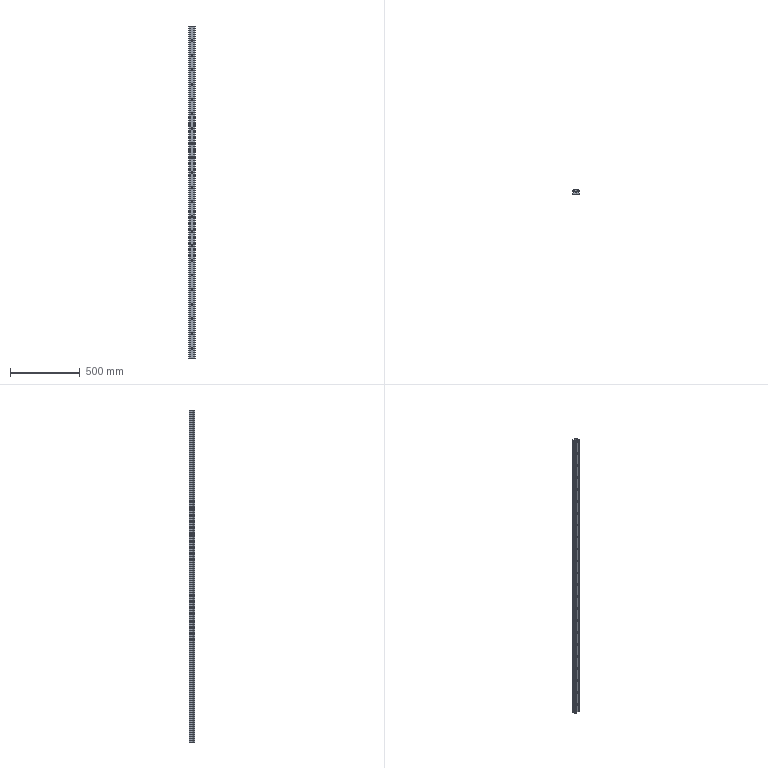Part | SolidWorks | features ICE 3, LPattern 2, BaseBody 1, RevCut 1 | 1 solid | 158 faces | box 45 x 38 x 2380 mm | volume 3190099 mm3 | cylinder 104 | plane 54 | commonest cylinder face diameters 14 x45 20 x45 2.4 x6 1.6 x4 8 x4